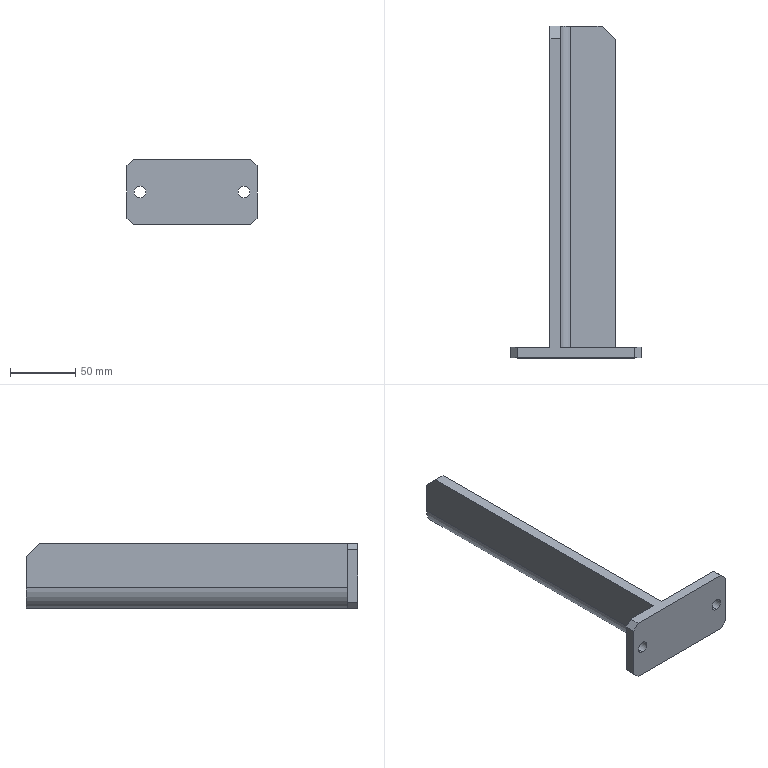Part | SolidWorks | features MBimport 1 | 1 solid | 24 faces | box 100 x 255 x 50 mm | volume 209397 mm3 | plane 18 | cylinder 6 | commonest cylinder face diameters 9 x4 16 x1 32 x1
STEP:
#1=CARTESIAN_POINT('',(-47.576,8.,-9.039));
#2=VERTEX_POINT('',#1);
#3=CARTESIAN_POINT('',(-42.576,8.,-4.039));
#4=VERTEX_POINT('',#3);
#5=CARTESIAN_POINT('',(-42.576,8.,-4.039));
#6=DIRECTION('',(0.7071,0.,0.7071));
#7=VECTOR('',#6,1000.);
#8=LINE('',#5,#7);
#9=EDGE_CURVE('',#2,#4,#8,.T.);
#10=ORIENTED_EDGE('',*,*,#9,.F.);
#11=CARTESIAN_POINT('',(-47.576,0.,-9.039));
#12=VERTEX_POINT('',#11);
#13=CARTESIAN_POINT('',(-47.576,8.,-9.039));
#14=DIRECTION('',(0.,1.,0.));
#15=VECTOR('',#14,1000.);
#16=LINE('',#13,#15);
#17=EDGE_CURVE('',#12,#2,#16,.T.);
#18=ORIENTED_EDGE('',*,*,#17,.F.);
#19=CARTESIAN_POINT('',(-42.576,0.,-4.039));
#20=VERTEX_POINT('',#19);
#21=CARTESIAN_POINT('',(-19.269,0.,19.269));
#22=DIRECTION('',(-0.7071,0.,-0.7071));
#23=VECTOR('',#22,1000.);
#24=LINE('',#21,#23);
#25=EDGE_CURVE('',#20,#12,#24,.T.);
#26=ORIENTED_EDGE('',*,*,#25,.F.);
#27=CARTESIAN_POINT('',(-42.576,8.,-4.039));
#28=DIRECTION('',(0.,-1.,0.));
#29=VECTOR('',#28,1000.);
#30=LINE('',#27,#29);
#31=EDGE_CURVE('',#4,#20,#30,.T.);
#32=ORIENTED_EDGE('',*,*,#31,.F.);
#33=EDGE_LOOP('',(#10,#18,#26,#32));
#34=FACE_OUTER_BOUND('',#33,.T.);
#35=CARTESIAN_POINT('',(-42.576,8.,-4.039));
#36=DIRECTION('',(0.7071,0.,-0.7071));
#37=DIRECTION('',(0.,-1.,0.));
#38=AXIS2_PLACEMENT_3D('',#35,#36,#37);
#39=PLANE('',#38);
#40=ADVANCED_FACE('',(#34),#39,.F.);
#41=CARTESIAN_POINT('',(47.424,8.,-4.039));
#42=VERTEX_POINT('',#41);
#43=CARTESIAN_POINT('',(52.424,8.,-9.039));
#44=VERTEX_POINT('',#43);
#45=CARTESIAN_POINT('',(52.424,8.,-9.039));
#46=DIRECTION('',(0.7071,0.,-0.7071));
#47=VECTOR('',#46,1000.);
#48=LINE('',#45,#47);
#49=EDGE_CURVE('',#42,#44,#48,.T.);
#50=ORIENTED_EDGE('',*,*,#49,.F.);
#51=CARTESIAN_POINT('',(47.424,0.,-4.039));
#52=VERTEX_POINT('',#51);
#53=CARTESIAN_POINT('',(47.424,8.,-4.039));
#54=DIRECTION('',(0.,1.,0.));
#55=VECTOR('',#54,1000.);
#56=LINE('',#53,#55);
#57=EDGE_CURVE('',#52,#42,#56,.T.);
#58=ORIENTED_EDGE('',*,*,#57,.F.);
#59=CARTESIAN_POINT('',(52.424,0.,-9.039));
#60=VERTEX_POINT('',#59);
#61=CARTESIAN_POINT('',(21.693,0.,21.693));
#62=DIRECTION('',(-0.7071,0.,0.7071));
#63=VECTOR('',#62,1000.);
#64=LINE('',#61,#63);
#65=EDGE_CURVE('',#60,#52,#64,.T.);
#66=ORIENTED_EDGE('',*,*,#65,.F.);
#67=CARTESIAN_POINT('',(52.424,8.,-9.039));
#68=DIRECTION('',(0.,-1.,0.));
#69=VECTOR('',#68,1000.);
#70=LINE('',#67,#69);
#71=EDGE_CURVE('',#44,#60,#70,.T.);
#72=ORIENTED_EDGE('',*,*,#71,.F.);
#73=EDGE_LOOP('',(#50,#58,#66,#72));
#74=FACE_OUTER_BOUND('',#73,.T.);
#75=CARTESIAN_POINT('',(52.424,8.,-9.039));
#76=DIRECTION('',(-0.7071,0.,-0.7071));
#77=DIRECTION('',(-0.7071,0.,0.7071));
#78=AXIS2_PLACEMENT_3D('',#75,#76,#77);
#79=PLANE('',#78);
#80=ADVANCED_FACE('',(#74),#79,.F.);
#81=CARTESIAN_POINT('',(52.424,8.,-49.039));
#82=VERTEX_POINT('',#81);
#83=CARTESIAN_POINT('',(47.424,8.,-54.039));
#84=VERTEX_POINT('',#83);
#85=CARTESIAN_POINT('',(47.424,8.,-54.039));
#86=DIRECTION('',(-0.7071,0.,-0.7071));
#87=VECTOR('',#86,1000.);
#88=LINE('',#85,#87);
#89=EDGE_CURVE('',#82,#84,#88,.T.);
#90=ORIENTED_EDGE('',*,*,#89,.F.);
#91=CARTESIAN_POINT('',(52.424,0.,-49.039));
#92=VERTEX_POINT('',#91);
#93=CARTESIAN_POINT('',(52.424,8.,-49.039));
#94=DIRECTION('',(0.,1.,0.));
#95=VECTOR('',#94,1000.);
#96=LINE('',#93,#95);
#97=EDGE_CURVE('',#92,#82,#96,.T.);
#98=ORIENTED_EDGE('',*,*,#97,.F.);
#99=CARTESIAN_POINT('',(47.424,0.,-54.039));
#100=VERTEX_POINT('',#99);
#101=CARTESIAN_POINT('',(50.731,0.,-50.731));
#102=DIRECTION('',(0.7071,0.,0.7071));
#103=VECTOR('',#102,1000.);
#104=LINE('',#101,#103);
#105=EDGE_CURVE('',#100,#92,#104,.T.);
#106=ORIENTED_EDGE('',*,*,#105,.F.);
#107=CARTESIAN_POINT('',(47.424,8.,-54.039));
#108=DIRECTION('',(0.,-1.,0.));
#109=VECTOR('',#108,1000.);
#110=LINE('',#107,#109);
#111=EDGE_CURVE('',#84,#100,#110,.T.);
#112=ORIENTED_EDGE('',*,*,#111,.F.);
#113=EDGE_LOOP('',(#90,#98,#106,#112));
#114=FACE_OUTER_BOUND('',#113,.T.);
#115=CARTESIAN_POINT('',(47.424,8.,-54.039));
#116=DIRECTION('',(-0.7071,0.,0.7071));
#117=DIRECTION('',(0.,1.,0.));
#118=AXIS2_PLACEMENT_3D('',#115,#116,#117);
#119=PLANE('',#118);
#120=ADVANCED_FACE('',(#114),#119,.F.);
#121=CARTESIAN_POINT('',(-42.576,8.,-54.039));
#122=VERTEX_POINT('',#121);
#123=CARTESIAN_POINT('',(-47.576,8.,-49.039));
#124=VERTEX_POINT('',#123);
#125=CARTESIAN_POINT('',(-47.576,8.,-49.039));
#126=DIRECTION('',(-0.7071,0.,0.7071));
#127=VECTOR('',#126,1000.);
#128=LINE('',#125,#127);
#129=EDGE_CURVE('',#122,#124,#128,.T.);
#130=ORIENTED_EDGE('',*,*,#129,.F.);
#131=CARTESIAN_POINT('',(-42.576,0.,-54.039));
#132=VERTEX_POINT('',#131);
#133=CARTESIAN_POINT('',(-42.576,8.,-54.039));
#134=DIRECTION('',(0.,1.,0.));
#135=VECTOR('',#134,1000.);
#136=LINE('',#133,#135);
#137=EDGE_CURVE('',#132,#122,#136,.T.);
#138=ORIENTED_EDGE('',*,*,#137,.F.);
#139=CARTESIAN_POINT('',(-47.576,0.,-49.039));
#140=VERTEX_POINT('',#139);
#141=CARTESIAN_POINT('',(-48.307,0.,-48.307));
#142=DIRECTION('',(0.7071,0.,-0.7071));
#143=VECTOR('',#142,1000.);
#144=LINE('',#141,#143);
#145=EDGE_CURVE('',#140,#132,#144,.T.);
#146=ORIENTED_EDGE('',*,*,#145,.F.);
#147=CARTESIAN_POINT('',(-47.576,8.,-49.039));
#148=DIRECTION('',(0.,-1.,0.));
#149=VECTOR('',#148,1000.);
#150=LINE('',#147,#149);
#151=EDGE_CURVE('',#124,#140,#150,.T.);
#152=ORIENTED_EDGE('',*,*,#151,.F.);
#153=EDGE_LOOP('',(#130,#138,#146,#152));
#154=FACE_OUTER_BOUND('',#153,.T.);
#155=CARTESIAN_POINT('',(-47.576,8.,-49.039));
#156=DIRECTION('',(0.7071,0.,0.7071));
#157=DIRECTION('',(0.,-1.,0.));
#158=AXIS2_PLACEMENT_3D('',#155,#156,#157);
#159=PLANE('',#158);
#160=ADVANCED_FACE('',(#154),#159,.F.);
#161=CARTESIAN_POINT('',(-17.576,245.,-4.039));
#162=VERTEX_POINT('',#161);
#163=CARTESIAN_POINT('',(-17.576,255.,-14.039));
#164=VERTEX_POINT('',#163);
#165=CARTESIAN_POINT('',(-17.576,255.,-14.039));
#166=DIRECTION('',(0.,0.7071,-0.7071));
#167=VECTOR('',#166,1000.);
#168=LINE('',#165,#167);
#169=EDGE_CURVE('',#162,#164,#168,.T.);
#170=ORIENTED_EDGE('',*,*,#169,.F.);
#171=CARTESIAN_POINT('',(-9.576,245.,-4.039));
#172=VERTEX_POINT('',#171);
#173=CARTESIAN_POINT('',(-47.576,245.,-4.039));
#174=DIRECTION('',(-1.,0.,0.));
#175=VECTOR('',#174,1000.);
#176=LINE('',#173,#175);
#177=EDGE_CURVE('',#172,#162,#176,.T.);
#178=ORIENTED_EDGE('',*,*,#177,.F.);
#179=CARTESIAN_POINT('',(-9.576,255.,-14.039));
#180=VERTEX_POINT('',#179);
#181=CARTESIAN_POINT('',(-9.576,255.,-14.039));
#182=DIRECTION('',(0.,-0.7071,0.7071));
#183=VECTOR('',#182,1000.);
#184=LINE('',#181,#183);
#185=EDGE_CURVE('',#180,#172,#184,.T.);
#186=ORIENTED_EDGE('',*,*,#185,.F.);
#187=CARTESIAN_POINT('',(-1.576,255.,-14.039));
#188=DIRECTION('',(1.,0.,0.));
#189=VECTOR('',#188,1000.);
#190=LINE('',#187,#189);
#191=EDGE_CURVE('',#164,#180,#190,.T.);
#192=ORIENTED_EDGE('',*,*,#191,.F.);
#193=EDGE_LOOP('',(#170,#178,#186,#192));
#194=FACE_OUTER_BOUND('',#193,.T.);
#195=CARTESIAN_POINT('',(-1.576,255.,-14.039));
#196=DIRECTION('',(0.,-0.7071,-0.7071));
#197=DIRECTION('',(0.,0.7071,-0.7071));
#198=AXIS2_PLACEMENT_3D('',#195,#196,#197);
#199=PLANE('',#198);
#200=ADVANCED_FACE('',(#194),#199,.F.);
#201=CARTESIAN_POINT('',(32.424,245.,-46.039));
#202=VERTEX_POINT('',#201);
#203=CARTESIAN_POINT('',(22.424,255.,-46.039));
#204=VERTEX_POINT('',#203);
#205=CARTESIAN_POINT('',(22.424,255.,-46.039));
#206=DIRECTION('',(-0.7071,0.7071,0.));
#207=VECTOR('',#206,1000.);
#208=LINE('',#205,#207);
#209=EDGE_CURVE('',#202,#204,#208,.T.);
#210=ORIENTED_EDGE('',*,*,#209,.F.);
#211=CARTESIAN_POINT('',(32.424,245.,-54.039));
#212=VERTEX_POINT('',#211);
#213=CARTESIAN_POINT('',(32.424,245.,-54.039));
#214=DIRECTION('',(0.,0.,1.));
#215=VECTOR('',#214,1000.);
#216=LINE('',#213,#215);
#217=EDGE_CURVE('',#212,#202,#216,.T.);
#218=ORIENTED_EDGE('',*,*,#217,.F.);
#219=CARTESIAN_POINT('',(22.424,255.,-54.039));
#220=VERTEX_POINT('',#219);
#221=CARTESIAN_POINT('',(22.424,255.,-54.039));
#222=DIRECTION('',(0.7071,-0.7071,0.));
#223=VECTOR('',#222,1000.);
#224=LINE('',#221,#223);
#225=EDGE_CURVE('',#220,#212,#224,.T.);
#226=ORIENTED_EDGE('',*,*,#225,.F.);
#227=CARTESIAN_POINT('',(22.424,255.,-38.039));
#228=DIRECTION('',(0.,0.,-1.));
#229=VECTOR('',#228,1000.);
#230=LINE('',#227,#229);
#231=EDGE_CURVE('',#204,#220,#230,.T.);
#232=ORIENTED_EDGE('',*,*,#231,.F.);
#233=EDGE_LOOP('',(#210,#218,#226,#232));
#234=FACE_OUTER_BOUND('',#233,.T.);
#235=CARTESIAN_POINT('',(22.424,255.,-38.039));
#236=DIRECTION('',(-0.7071,-0.7071,0.));
#237=DIRECTION('',(-0.7071,0.7071,0.));
#238=AXIS2_PLACEMENT_3D('',#235,#236,#237);
#239=PLANE('',#238);
#240=ADVANCED_FACE('',(#234),#239,.F.);
#241=CARTESIAN_POINT('',(-1.576,255.,-46.039));
#242=VERTEX_POINT('',#241);
#243=CARTESIAN_POINT('',(-1.576,255.,-46.039));
#244=DIRECTION('',(1.,0.,0.));
#245=VECTOR('',#244,1000.);
#246=LINE('',#243,#245);
#247=EDGE_CURVE('',#242,#204,#246,.T.);
#248=ORIENTED_EDGE('',*,*,#247,.T.);
#249=ORIENTED_EDGE('',*,*,#231,.T.);
#250=CARTESIAN_POINT('',(-1.576,255.,-54.039));
#251=VERTEX_POINT('',#250);
#252=CARTESIAN_POINT('',(-1.576,255.,-54.039));
#253=DIRECTION('',(-1.,0.,0.));
#254=VECTOR('',#253,1000.);
#255=LINE('',#252,#254);
#256=EDGE_CURVE('',#220,#251,#255,.T.);
#257=ORIENTED_EDGE('',*,*,#256,.T.);
#258=CARTESIAN_POINT('',(-17.576,255.,-38.039));
#259=VERTEX_POINT('',#258);
#260=CARTESIAN_POINT('',(-1.576,255.,-38.039));
#261=DIRECTION('',(0.,1.,0.));
#262=DIRECTION('',(0.,0.,-1.));
#263=AXIS2_PLACEMENT_3D('',#260,#261,#262);
#264=CIRCLE('',#263,16.);
#265=EDGE_CURVE('',#251,#259,#264,.T.);
#266=ORIENTED_EDGE('',*,*,#265,.T.);
#267=CARTESIAN_POINT('',(-17.576,255.,-4.039));
#268=DIRECTION('',(0.,0.,1.));
#269=VECTOR('',#268,1000.);
#270=LINE('',#267,#269);
#271=EDGE_CURVE('',#259,#164,#270,.T.);
#272=ORIENTED_EDGE('',*,*,#271,.T.);
#273=ORIENTED_EDGE('',*,*,#191,.T.);
#274=CARTESIAN_POINT('',(-9.576,255.,-38.039));
#275=VERTEX_POINT('',#274);
#276=CARTESIAN_POINT('',(-9.576,255.,-4.039));
#277=DIRECTION('',(0.,0.,-1.));
#278=VECTOR('',#277,1000.);
#279=LINE('',#276,#278);
#280=EDGE_CURVE('',#180,#275,#279,.T.);
#281=ORIENTED_EDGE('',*,*,#280,.T.);
#282=CARTESIAN_POINT('',(-1.576,255.,-38.039));
#283=DIRECTION('',(0.,-1.,0.));
#284=DIRECTION('',(0.,0.,-1.));
#285=AXIS2_PLACEMENT_3D('',#282,#283,#284);
#286=CIRCLE('',#285,8.);
#287=EDGE_CURVE('',#275,#242,#286,.T.);
#288=ORIENTED_EDGE('',*,*,#287,.T.);
#289=EDGE_LOOP('',(#248,#249,#257,#266,#272,#273,#281,#288));
#290=FACE_OUTER_BOUND('',#289,.T.);
#291=CARTESIAN_POINT('',(-1.576,255.,-38.039));
#292=DIRECTION('',(0.,-1.,0.));
#293=DIRECTION('',(0.,0.,-1.));
#294=AXIS2_PLACEMENT_3D('',#291,#292,#293);
#295=PLANE('',#294);
#296=ADVANCED_FACE('',(#290),#295,.F.);
#297=CARTESIAN_POINT('',(-17.576,8.,-4.039));
#298=VERTEX_POINT('',#297);
#299=CARTESIAN_POINT('',(-17.576,255.,-4.039));
#300=DIRECTION('',(0.,-1.,0.));
#301=VECTOR('',#300,1000.);
#302=LINE('',#299,#301);
#303=EDGE_CURVE('',#162,#298,#302,.T.);
#304=ORIENTED_EDGE('',*,*,#303,.F.);
#305=ORIENTED_EDGE('',*,*,#169,.T.);
#306=ORIENTED_EDGE('',*,*,#271,.F.);
#307=CARTESIAN_POINT('',(-17.576,8.,-38.039));
#308=VERTEX_POINT('',#307);
#309=CARTESIAN_POINT('',(-17.576,255.,-38.039));
#310=DIRECTION('',(0.,-1.,0.));
#311=VECTOR('',#310,1000.);
#312=LINE('',#309,#311);
#313=EDGE_CURVE('',#259,#308,#312,.T.);
#314=ORIENTED_EDGE('',*,*,#313,.T.);
#315=CARTESIAN_POINT('',(-17.576,8.,-4.039));
#316=DIRECTION('',(0.,0.,1.));
#317=VECTOR('',#316,1000.);
#318=LINE('',#315,#317);
#319=EDGE_CURVE('',#308,#298,#318,.T.);
#320=ORIENTED_EDGE('',*,*,#319,.T.);
#321=EDGE_LOOP('',(#304,#305,#306,#314,#320));
#322=FACE_OUTER_BOUND('',#321,.T.);
#323=CARTESIAN_POINT('',(-17.576,255.,-4.039));
#324=DIRECTION('',(1.,0.,0.));
#325=DIRECTION('',(0.,0.,-1.));
#326=AXIS2_PLACEMENT_3D('',#323,#324,#325);
#327=PLANE('',#326);
#328=ADVANCED_FACE('',(#322),#327,.F.);
#329=CARTESIAN_POINT('',(-1.576,8.,-54.039));
#330=VERTEX_POINT('',#329);
#331=CARTESIAN_POINT('',(-1.576,8.,-38.039));
#332=DIRECTION('',(0.,1.,0.));
#333=DIRECTION('',(0.,0.,-1.));
#334=AXIS2_PLACEMENT_3D('',#331,#332,#333);
#335=CIRCLE('',#334,16.);
#336=EDGE_CURVE('',#330,#308,#335,.T.);
#337=ORIENTED_EDGE('',*,*,#336,.T.);
#338=ORIENTED_EDGE('',*,*,#313,.F.);
#339=ORIENTED_EDGE('',*,*,#265,.F.);
#340=CARTESIAN_POINT('',(-1.576,255.,-54.039));
#341=DIRECTION('',(0.,-1.,0.));
#342=VECTOR('',#341,1000.);
#343=LINE('',#340,#342);
#344=EDGE_CURVE('',#251,#330,#343,.T.);
#345=ORIENTED_EDGE('',*,*,#344,.T.);
#346=EDGE_LOOP('',(#337,#338,#339,#345));
#347=FACE_OUTER_BOUND('',#346,.T.);
#348=CARTESIAN_POINT('',(-1.576,255.,-38.039));
#349=DIRECTION('',(0.,-1.,0.));
#350=DIRECTION('',(0.,0.,-1.));
#351=AXIS2_PLACEMENT_3D('',#348,#349,#350);
#352=CYLINDRICAL_SURFACE('',#351,16.);
#353=ADVANCED_FACE('',(#347),#352,.T.);
#354=CARTESIAN_POINT('',(32.424,8.,-54.039));
#355=VERTEX_POINT('',#354);
#356=CARTESIAN_POINT('',(32.424,255.,-54.039));
#357=DIRECTION('',(0.,-1.,0.));
#358=VECTOR('',#357,1000.);
#359=LINE('',#356,#358);
#360=EDGE_CURVE('',#212,#355,#359,.T.);
#361=ORIENTED_EDGE('',*,*,#360,.F.);
#362=ORIENTED_EDGE('',*,*,#217,.T.);
#363=CARTESIAN_POINT('',(32.424,8.,-46.039));
#364=VERTEX_POINT('',#363);
#365=CARTESIAN_POINT('',(32.424,255.,-46.039));
#366=DIRECTION('',(0.,-1.,0.));
#367=VECTOR('',#366,1000.);
#368=LINE('',#365,#367);
#369=EDGE_CURVE('',#202,#364,#368,.T.);
#370=ORIENTED_EDGE('',*,*,#369,.T.);
#371=CARTESIAN_POINT('',(32.424,8.,-54.039));
#372=DIRECTION('',(0.,0.,-1.));
#373=VECTOR('',#372,1000.);
#374=LINE('',#371,#373);
#375=EDGE_CURVE('',#364,#355,#374,.T.);
#376=ORIENTED_EDGE('',*,*,#375,.T.);
#377=EDGE_LOOP('',(#361,#362,#370,#376));
#378=FACE_OUTER_BOUND('',#377,.T.);
#379=CARTESIAN_POINT('',(32.424,255.,-54.039));
#380=DIRECTION('',(-1.,0.,0.));
#381=DIRECTION('',(0.,0.,1.));
#382=AXIS2_PLACEMENT_3D('',#379,#380,#381);
#383=PLANE('',#382);
#384=ADVANCED_FACE('',(#378),#383,.F.);
#385=ORIENTED_EDGE('',*,*,#369,.F.);
#386=ORIENTED_EDGE('',*,*,#209,.T.);
#387=ORIENTED_EDGE('',*,*,#247,.F.);
#388=CARTESIAN_POINT('',(-1.576,8.,-46.039));
#389=VERTEX_POINT('',#388);
#390=CARTESIAN_POINT('',(-1.576,255.,-46.039));
#391=DIRECTION('',(0.,-1.,0.));
#392=VECTOR('',#391,1000.);
#393=LINE('',#390,#392);
#394=EDGE_CURVE('',#242,#389,#393,.T.);
#395=ORIENTED_EDGE('',*,*,#394,.T.);
#396=CARTESIAN_POINT('',(-1.576,8.,-46.039));
#397=DIRECTION('',(1.,0.,0.));
#398=VECTOR('',#397,1000.);
#399=LINE('',#396,#398);
#400=EDGE_CURVE('',#389,#364,#399,.T.);
#401=ORIENTED_EDGE('',*,*,#400,.T.);
#402=EDGE_LOOP('',(#385,#386,#387,#395,#401));
#403=FACE_OUTER_BOUND('',#402,.T.);
#404=CARTESIAN_POINT('',(-1.576,255.,-46.039));
#405=DIRECTION('',(0.,0.,-1.));
#406=DIRECTION('',(0.,-1.,0.));
#407=AXIS2_PLACEMENT_3D('',#404,#405,#406);
#408=PLANE('',#407);
#409=ADVANCED_FACE('',(#403),#408,.F.);
#410=CARTESIAN_POINT('',(-9.576,8.,-38.039));
#411=VERTEX_POINT('',#410);
#412=CARTESIAN_POINT('',(-1.576,8.,-38.039));
#413=DIRECTION('',(0.,-1.,0.));
#414=DIRECTION('',(0.,0.,-1.));
#415=AXIS2_PLACEMENT_3D('',#412,#413,#414);
#416=CIRCLE('',#415,8.);
#417=EDGE_CURVE('',#411,#389,#416,.T.);
#418=ORIENTED_EDGE('',*,*,#417,.T.);
#419=ORIENTED_EDGE('',*,*,#394,.F.);
#420=ORIENTED_EDGE('',*,*,#287,.F.);
#421=CARTESIAN_POINT('',(-9.576,255.,-38.039));
#422=DIRECTION('',(0.,-1.,0.));
#423=VECTOR('',#422,1000.);
#424=LINE('',#421,#423);
#425=EDGE_CURVE('',#275,#411,#424,.T.);
#426=ORIENTED_EDGE('',*,*,#425,.T.);
#427=EDGE_LOOP('',(#418,#419,#420,#426));
#428=FACE_OUTER_BOUND('',#427,.T.);
#429=CARTESIAN_POINT('',(-1.576,255.,-38.039));
#430=DIRECTION('',(0.,-1.,0.));
#431=DIRECTION('',(0.,0.,-1.));
#432=AXIS2_PLACEMENT_3D('',#429,#430,#431);
#433=CYLINDRICAL_SURFACE('',#432,8.);
#434=ADVANCED_FACE('',(#428),#433,.F.);
#435=ORIENTED_EDGE('',*,*,#280,.F.);
#436=ORIENTED_EDGE('',*,*,#185,.T.);
#437=CARTESIAN_POINT('',(-9.576,8.,-4.039));
#438=VERTEX_POINT('',#437);
#439=CARTESIAN_POINT('',(-9.576,255.,-4.039));
#440=DIRECTION('',(0.,-1.,0.));
#441=VECTOR('',#440,1000.);
#442=LINE('',#439,#441);
#443=EDGE_CURVE('',#172,#438,#442,.T.);
#444=ORIENTED_EDGE('',*,*,#443,.T.);
#445=CARTESIAN_POINT('',(-9.576,8.,-4.039));
#446=DIRECTION('',(0.,0.,-1.));
#447=VECTOR('',#446,1000.);
#448=LINE('',#445,#447);
#449=EDGE_CURVE('',#438,#411,#448,.T.);
#450=ORIENTED_EDGE('',*,*,#449,.T.);
#451=ORIENTED_EDGE('',*,*,#425,.F.);
#452=EDGE_LOOP('',(#435,#436,#444,#450,#451));
#453=FACE_OUTER_BOUND('',#452,.T.);
#454=CARTESIAN_POINT('',(-9.576,255.,-4.039));
#455=DIRECTION('',(-1.,0.,0.));
#456=DIRECTION('',(0.,1.,0.));
#457=AXIS2_PLACEMENT_3D('',#454,#455,#456);
#458=PLANE('',#457);
#459=ADVANCED_FACE('',(#453),#458,.F.);
#460=CARTESIAN_POINT('',(42.424,8.,-24.539));
#461=VERTEX_POINT('',#460);
#462=CARTESIAN_POINT('',(42.424,0.,-24.539));
#463=VERTEX_POINT('',#462);
#464=CARTESIAN_POINT('',(42.424,8.,-24.539));
#465=DIRECTION('',(0.,-1.,0.));
#466=VECTOR('',#465,1000.);
#467=LINE('',#464,#466);
#468=EDGE_CURVE('',#461,#463,#467,.T.);
#469=ORIENTED_EDGE('',*,*,#468,.F.);
#470=CARTESIAN_POINT('',(42.424,8.,-33.539));
#471=VERTEX_POINT('',#470);
#472=CARTESIAN_POINT('',(42.424,8.,-29.039));
#473=DIRECTION('',(0.,1.,0.));
#474=DIRECTION('',(0.,0.,1.));
#475=AXIS2_PLACEMENT_3D('',#472,#473,#474);
#476=CIRCLE('',#475,4.5);
#477=EDGE_CURVE('',#461,#471,#476,.T.);
#478=ORIENTED_EDGE('',*,*,#477,.T.);
#479=CARTESIAN_POINT('',(42.424,0.,-33.539));
#480=VERTEX_POINT('',#479);
#481=CARTESIAN_POINT('',(42.424,8.,-33.539));
#482=DIRECTION('',(0.,-1.,0.));
#483=VECTOR('',#482,1000.);
#484=LINE('',#481,#483);
#485=EDGE_CURVE('',#471,#480,#484,.T.);
#486=ORIENTED_EDGE('',*,*,#485,.T.);
#487=CARTESIAN_POINT('',(42.424,0.,-29.039));
#488=DIRECTION('',(0.,1.,0.));
#489=DIRECTION('',(0.,0.,1.));
#490=AXIS2_PLACEMENT_3D('',#487,#488,#489);
#491=CIRCLE('',#490,4.5);
#492=EDGE_CURVE('',#463,#480,#491,.T.);
#493=ORIENTED_EDGE('',*,*,#492,.F.);
#494=EDGE_LOOP('',(#469,#478,#486,#493));
#495=FACE_OUTER_BOUND('',#494,.T.);
#496=CARTESIAN_POINT('',(42.424,8.,-29.039));
#497=DIRECTION('',(0.,-1.,0.));
#498=DIRECTION('',(0.,0.,-1.));
#499=AXIS2_PLACEMENT_3D('',#496,#497,#498);
#500=CYLINDRICAL_SURFACE('',#499,4.5);
#501=ADVANCED_FACE('',(#495),#500,.F.);
#502=CARTESIAN_POINT('',(-37.576,8.,-24.539));
#503=VERTEX_POINT('',#502);
#504=CARTESIAN_POINT('',(-37.576,0.,-24.539));
#505=VERTEX_POINT('',#504);
#506=CARTESIAN_POINT('',(-37.576,8.,-24.539));
#507=DIRECTION('',(0.,-1.,0.));
#508=VECTOR('',#507,1000.);
#509=LINE('',#506,#508);
#510=EDGE_CURVE('',#503,#505,#509,.T.);
#511=ORIENTED_EDGE('',*,*,#510,.F.);
#512=CARTESIAN_POINT('',(-37.576,8.,-33.539));
#513=VERTEX_POINT('',#512);
#514=CARTESIAN_POINT('',(-37.576,8.,-29.039));
#515=DIRECTION('',(0.,1.,0.));
#516=DIRECTION('',(0.,0.,1.));
#517=AXIS2_PLACEMENT_3D('',#514,#515,#516);
#518=CIRCLE('',#517,4.5);
#519=EDGE_CURVE('',#503,#513,#518,.T.);
#520=ORIENTED_EDGE('',*,*,#519,.T.);
#521=CARTESIAN_POINT('',(-37.576,0.,-33.539));
#522=VERTEX_POINT('',#521);
#523=CARTESIAN_POINT('',(-37.576,8.,-33.539));
#524=DIRECTION('',(0.,-1.,0.));
#525=VECTOR('',#524,1000.);
#526=LINE('',#523,#525);
#527=EDGE_CURVE('',#513,#522,#526,.T.);
#528=ORIENTED_EDGE('',*,*,#527,.T.);
#529=CARTESIAN_POINT('',(-37.576,0.,-29.039));
#530=DIRECTION('',(0.,1.,0.));
#531=DIRECTION('',(0.,0.,1.));
#532=AXIS2_PLACEMENT_3D('',#529,#530,#531);
#533=CIRCLE('',#532,4.5);
#534=EDGE_CURVE('',#505,#522,#533,.T.);
#535=ORIENTED_EDGE('',*,*,#534,.F.);
#536=EDGE_LOOP('',(#511,#520,#528,#535));
#537=FACE_OUTER_BOUND('',#536,.T.);
#538=CARTESIAN_POINT('',(-37.576,8.,-29.039));
#539=DIRECTION('',(0.,-1.,0.));
#540=DIRECTION('',(0.,0.,-1.));
#541=AXIS2_PLACEMENT_3D('',#538,#539,#540);
#542=CYLINDRICAL_SURFACE('',#541,4.5);
#543=ADVANCED_FACE('',(#537),#542,.F.);
#544=CARTESIAN_POINT('',(-47.576,0.,-54.039));
#545=DIRECTION('',(-1.,0.,0.));
#546=VECTOR('',#545,1000.);
#547=LINE('',#544,#546);
#548=EDGE_CURVE('',#100,#132,#547,.T.);
#549=ORIENTED_EDGE('',*,*,#548,.T.);
#550=ORIENTED_EDGE('',*,*,#137,.T.);
#551=CARTESIAN_POINT('',(-47.576,8.,-54.039));
#552=DIRECTION('',(-1.,0.,0.));
#553=VECTOR('',#552,1000.);
#554=LINE('',#551,#553);
#555=EDGE_CURVE('',#330,#122,#554,.T.);
#556=ORIENTED_EDGE('',*,*,#555,.F.);
#557=ORIENTED_EDGE('',*,*,#344,.F.);
#558=ORIENTED_EDGE('',*,*,#256,.F.);
#559=ORIENTED_EDGE('',*,*,#225,.T.);
#560=ORIENTED_EDGE('',*,*,#360,.T.);
#561=CARTESIAN_POINT('',(-47.576,8.,-54.039));
#562=DIRECTION('',(-1.,0.,0.));
#563=VECTOR('',#562,1000.);
#564=LINE('',#561,#563);
#565=EDGE_CURVE('',#84,#355,#564,.T.);
#566=ORIENTED_EDGE('',*,*,#565,.F.);
#567=ORIENTED_EDGE('',*,*,#111,.T.);
#568=EDGE_LOOP('',(#549,#550,#556,#557,#558,#559,#560,#566,#567));
#569=FACE_OUTER_BOUND('',#568,.T.);
#570=CARTESIAN_POINT('',(-47.576,8.,-54.039));
#571=DIRECTION('',(0.,0.,1.));
#572=DIRECTION('',(1.,0.,0.));
#573=AXIS2_PLACEMENT_3D('',#570,#571,#572);
#574=PLANE('',#573);
#575=ADVANCED_FACE('',(#569),#574,.F.);
#576=CARTESIAN_POINT('',(52.424,0.,-4.039));
#577=DIRECTION('',(0.,0.,-1.));
#578=VECTOR('',#577,1000.);
#579=LINE('',#576,#578);
#580=EDGE_CURVE('',#60,#92,#579,.T.);
#581=ORIENTED_EDGE('',*,*,#580,.T.);
#582=ORIENTED_EDGE('',*,*,#97,.T.);
#583=CARTESIAN_POINT('',(52.424,8.,-4.039));
#584=DIRECTION('',(0.,0.,-1.));
#585=VECTOR('',#584,1000.);
#586=LINE('',#583,#585);
#587=EDGE_CURVE('',#44,#82,#586,.T.);
#588=ORIENTED_EDGE('',*,*,#587,.F.);
#589=ORIENTED_EDGE('',*,*,#71,.T.);
#590=EDGE_LOOP('',(#581,#582,#588,#589));
#591=FACE_OUTER_BOUND('',#590,.T.);
#592=CARTESIAN_POINT('',(52.424,8.,-4.039));
#593=DIRECTION('',(-1.,0.,0.));
#594=DIRECTION('',(0.,0.,1.));
#595=AXIS2_PLACEMENT_3D('',#592,#593,#594);
#596=PLANE('',#595);
#597=ADVANCED_FACE('',(#591),#596,.F.);
#598=CARTESIAN_POINT('',(-47.576,0.,-4.039));
#599=DIRECTION('',(1.,0.,0.));
#600=VECTOR('',#599,1000.);
#601=LINE('',#598,#600);
#602=EDGE_CURVE('',#20,#52,#601,.T.);
#603=ORIENTED_EDGE('',*,*,#602,.T.);
#604=ORIENTED_EDGE('',*,*,#57,.T.);
#605=CARTESIAN_POINT('',(-47.576,8.,-4.039));
#606=DIRECTION('',(1.,0.,0.));
#607=VECTOR('',#606,1000.);
#608=LINE('',#605,#607);
#609=EDGE_CURVE('',#438,#42,#608,.T.);
#610=ORIENTED_EDGE('',*,*,#609,.F.);
#611=ORIENTED_EDGE('',*,*,#443,.F.);
#612=ORIENTED_EDGE('',*,*,#177,.T.);
#613=ORIENTED_EDGE('',*,*,#303,.T.);
#614=CARTESIAN_POINT('',(-47.576,8.,-4.039));
#615=DIRECTION('',(1.,0.,0.));
#616=VECTOR('',#615,1000.);
#617=LINE('',#614,#616);
#618=EDGE_CURVE('',#4,#298,#617,.T.);
#619=ORIENTED_EDGE('',*,*,#618,.F.);
#620=ORIENTED_EDGE('',*,*,#31,.T.);
#621=EDGE_LOOP('',(#603,#604,#610,#611,#612,#613,#619,#620));
#622=FACE_OUTER_BOUND('',#621,.T.);
#623=CARTESIAN_POINT('',(-47.576,8.,-4.039));
#624=DIRECTION('',(0.,0.,-1.));
#625=DIRECTION('',(0.,-1.,0.));
#626=AXIS2_PLACEMENT_3D('',#623,#624,#625);
#627=PLANE('',#626);
#628=ADVANCED_FACE('',(#622),#627,.F.);
#629=CARTESIAN_POINT('',(-47.576,8.,-4.039));
#630=DIRECTION('',(0.,0.,1.));
#631=VECTOR('',#630,1000.);
#632=LINE('',#629,#631);
#633=EDGE_CURVE('',#124,#2,#632,.T.);
#634=ORIENTED_EDGE('',*,*,#633,.F.);
#635=ORIENTED_EDGE('',*,*,#151,.T.);
#636=CARTESIAN_POINT('',(-47.576,0.,-4.039));
#637=DIRECTION('',(0.,0.,1.));
#638=VECTOR('',#637,1000.);
#639=LINE('',#636,#638);
#640=EDGE_CURVE('',#140,#12,#639,.T.);
#641=ORIENTED_EDGE('',*,*,#640,.T.);
#642=ORIENTED_EDGE('',*,*,#17,.T.);
#643=EDGE_LOOP('',(#634,#635,#641,#642));
#644=FACE_OUTER_BOUND('',#643,.T.);
#645=CARTESIAN_POINT('',(-47.576,8.,-4.039));
#646=DIRECTION('',(1.,0.,0.));
#647=DIRECTION('',(0.,1.,0.));
#648=AXIS2_PLACEMENT_3D('',#645,#646,#647);
#649=PLANE('',#648);
#650=ADVANCED_FACE('',(#644),#649,.F.);
#651=CARTESIAN_POINT('',(42.424,0.,-29.039));
#652=DIRECTION('',(0.,1.,0.));
#653=DIRECTION('',(0.,0.,1.));
#654=AXIS2_PLACEMENT_3D('',#651,#652,#653);
#655=CIRCLE('',#654,4.5);
#656=EDGE_CURVE('',#480,#463,#655,.T.);
#657=ORIENTED_EDGE('',*,*,#656,.T.);
#658=ORIENTED_EDGE('',*,*,#492,.T.);
#659=EDGE_LOOP('',(#657,#658));
#660=FACE_BOUND('',#659,.T.);
#661=CARTESIAN_POINT('',(-37.576,0.,-29.039));
#662=DIRECTION('',(0.,1.,0.));
#663=DIRECTION('',(0.,0.,1.));
#664=AXIS2_PLACEMENT_3D('',#661,#662,#663);
#665=CIRCLE('',#664,4.5);
#666=EDGE_CURVE('',#522,#505,#665,.T.);
#667=ORIENTED_EDGE('',*,*,#666,.T.);
#668=ORIENTED_EDGE('',*,*,#534,.T.);
#669=EDGE_LOOP('',(#667,#668));
#670=FACE_BOUND('',#669,.T.);
#671=ORIENTED_EDGE('',*,*,#640,.F.);
#672=ORIENTED_EDGE('',*,*,#145,.T.);
#673=ORIENTED_EDGE('',*,*,#548,.F.);
#674=ORIENTED_EDGE('',*,*,#105,.T.);
#675=ORIENTED_EDGE('',*,*,#580,.F.);
#676=ORIENTED_EDGE('',*,*,#65,.T.);
#677=ORIENTED_EDGE('',*,*,#602,.F.);
#678=ORIENTED_EDGE('',*,*,#25,.T.);
#679=EDGE_LOOP('',(#671,#672,#673,#674,#675,#676,#677,#678));
#680=FACE_OUTER_BOUND('',#679,.T.);
#681=CARTESIAN_POINT('',(0.,0.,0.));
#682=DIRECTION('',(0.,-1.,0.));
#683=DIRECTION('',(0.,0.,-1.));
#684=AXIS2_PLACEMENT_3D('',#681,#682,#683);
#685=PLANE('',#684);
#686=ADVANCED_FACE('',(#660,#670,#680),#685,.T.);
#687=CARTESIAN_POINT('',(42.424,8.,-29.039));
#688=DIRECTION('',(0.,1.,0.));
#689=DIRECTION('',(0.,0.,1.));
#690=AXIS2_PLACEMENT_3D('',#687,#688,#689);
#691=CIRCLE('',#690,4.5);
#692=EDGE_CURVE('',#471,#461,#691,.T.);
#693=ORIENTED_EDGE('',*,*,#692,.F.);
#694=ORIENTED_EDGE('',*,*,#477,.F.);
#695=EDGE_LOOP('',(#693,#694));
#696=FACE_BOUND('',#695,.T.);
#697=ORIENTED_EDGE('',*,*,#587,.T.);
#698=ORIENTED_EDGE('',*,*,#89,.T.);
#699=ORIENTED_EDGE('',*,*,#565,.T.);
#700=ORIENTED_EDGE('',*,*,#375,.F.);
#701=ORIENTED_EDGE('',*,*,#400,.F.);
#702=ORIENTED_EDGE('',*,*,#417,.F.);
#703=ORIENTED_EDGE('',*,*,#449,.F.);
#704=ORIENTED_EDGE('',*,*,#609,.T.);
#705=ORIENTED_EDGE('',*,*,#49,.T.);
#706=EDGE_LOOP('',(#697,#698,#699,#700,#701,#702,#703,#704,#705));
#707=FACE_OUTER_BOUND('',#706,.T.);
#708=CARTESIAN_POINT('',(0.,8.,0.));
#709=DIRECTION('',(0.,-1.,0.));
#710=DIRECTION('',(0.,0.,-1.));
#711=AXIS2_PLACEMENT_3D('',#708,#709,#710);
#712=PLANE('',#711);
#713=ADVANCED_FACE('',(#696,#707),#712,.F.);
#714=CARTESIAN_POINT('',(-37.576,8.,-29.039));
#715=DIRECTION('',(0.,1.,0.));
#716=DIRECTION('',(0.,0.,1.));
#717=AXIS2_PLACEMENT_3D('',#714,#715,#716);
#718=CIRCLE('',#717,4.5);
#719=EDGE_CURVE('',#513,#503,#718,.T.);
#720=ORIENTED_EDGE('',*,*,#719,.F.);
#721=ORIENTED_EDGE('',*,*,#519,.F.);
#722=EDGE_LOOP('',(#720,#721));
#723=FACE_BOUND('',#722,.T.);
#724=ORIENTED_EDGE('',*,*,#555,.T.);
#725=ORIENTED_EDGE('',*,*,#129,.T.);
#726=ORIENTED_EDGE('',*,*,#633,.T.);
#727=ORIENTED_EDGE('',*,*,#9,.T.);
#728=ORIENTED_EDGE('',*,*,#618,.T.);
#729=ORIENTED_EDGE('',*,*,#319,.F.);
#730=ORIENTED_EDGE('',*,*,#336,.F.);
#731=EDGE_LOOP('',(#724,#725,#726,#727,#728,#729,#730));
#732=FACE_OUTER_BOUND('',#731,.T.);
#733=CARTESIAN_POINT('',(0.,8.,0.));
#734=DIRECTION('',(0.,-1.,0.));
#735=DIRECTION('',(0.,0.,-1.));
#736=AXIS2_PLACEMENT_3D('',#733,#734,#735);
#737=PLANE('',#736);
#738=ADVANCED_FACE('',(#723,#732),#737,.F.);
#739=ORIENTED_EDGE('',*,*,#719,.T.);
#740=ORIENTED_EDGE('',*,*,#510,.T.);
#741=ORIENTED_EDGE('',*,*,#666,.F.);
#742=ORIENTED_EDGE('',*,*,#527,.F.);
#743=EDGE_LOOP('',(#739,#740,#741,#742));
#744=FACE_OUTER_BOUND('',#743,.T.);
#745=CARTESIAN_POINT('',(-37.576,8.,-29.039));
#746=DIRECTION('',(0.,-1.,0.));
#747=DIRECTION('',(0.,0.,-1.));
#748=AXIS2_PLACEMENT_3D('',#745,#746,#747);
#749=CYLINDRICAL_SURFACE('',#748,4.5);
#750=ADVANCED_FACE('',(#744),#749,.F.);
#751=ORIENTED_EDGE('',*,*,#692,.T.);
#752=ORIENTED_EDGE('',*,*,#468,.T.);
#753=ORIENTED_EDGE('',*,*,#656,.F.);
#754=ORIENTED_EDGE('',*,*,#485,.F.);
#755=EDGE_LOOP('',(#751,#752,#753,#754));
#756=FACE_OUTER_BOUND('',#755,.T.);
#757=CARTESIAN_POINT('',(42.424,8.,-29.039));
#758=DIRECTION('',(0.,-1.,0.));
#759=DIRECTION('',(0.,0.,-1.));
#760=AXIS2_PLACEMENT_3D('',#757,#758,#759);
#761=CYLINDRICAL_SURFACE('',#760,4.5);
#762=ADVANCED_FACE('',(#756),#761,.F.);
#763=CLOSED_SHELL('',(#40,#80,#120,#160,#200,#240,#296,#328,#353,#384,#409,#434,#459,#501,#543,#575,#597,#628,#650,#686,#713,#738,#750,#762));
#764=MANIFOLD_SOLID_BREP('',#763);
#765=CARTESIAN_POINT('',(0.,0.,0.));
#766=DIRECTION('',(0.,0.,1.));
#767=DIRECTION('',(1.,0.,0.));
#768=AXIS2_PLACEMENT_3D('',#765,#766,#767);
#769=(LENGTH_UNIT()NAMED_UNIT(*)SI_UNIT(.MILLI.,.METRE.));
#770=UNCERTAINTY_MEASURE_WITH_UNIT(LENGTH_MEASURE(0.00001),#769,'','');
#771=(NAMED_UNIT(*)PLANE_ANGLE_UNIT()SI_UNIT($,.RADIAN.));
#772=(NAMED_UNIT(*)SI_UNIT($,.STERADIAN.)SOLID_ANGLE_UNIT());
#773=(GEOMETRIC_REPRESENTATION_CONTEXT(3)GLOBAL_UNCERTAINTY_ASSIGNED_CONTEXT((#770))GLOBAL_UNIT_ASSIGNED_CONTEXT((#769,#771,#772))REPRESENTATION_CONTEXT('',''));
#774=ADVANCED_BREP_SHAPE_REPRESENTATION('',(#764,#768),#773);